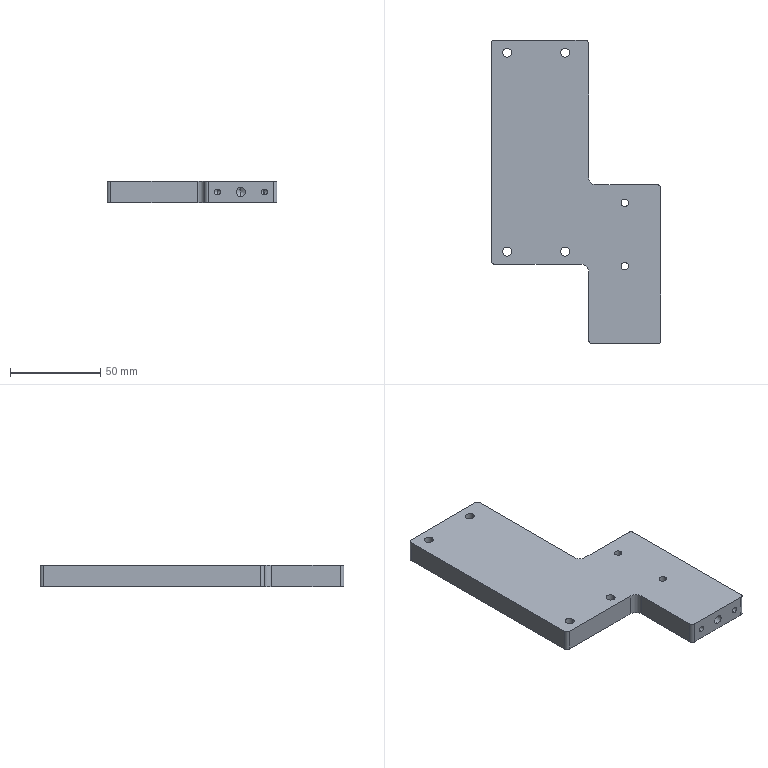Part | STEP file | 1 solid | 42 faces | box 94 x 168 x 12 mm | volume 120953 mm3 | cylinder 26 | plane 10 | cone 6 | commonest cylinder face diameters 5 x10 4 x6 3.3 x4 4.2 x4 8 x2